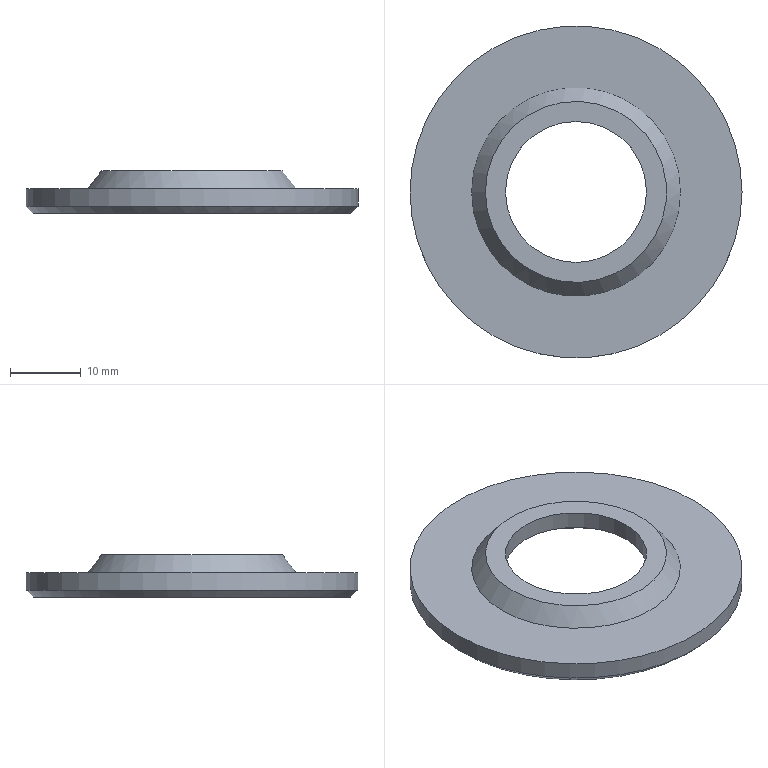Part | NX | features DATUM_CSYS 2, CHAMFER 1, SKETCH 1, SWP104 1 | 1 solid | 9 faces | box 47.08 x 47.08 x 6 mm | volume 4835 mm3 | plane 4 | cone 3 | cylinder 2 | commonest cylinder face diameters 20 x1 47.08 x1
STEP:
#1=CARTESIAN_POINT('',(-10.,0.,0.));
#2=VERTEX_POINT('',#1);
#3=CARTESIAN_POINT('',(0.,0.,0.));
#4=DIRECTION('',(0.,0.,-1.));
#5=DIRECTION('',(-1.,0.,0.));
#6=AXIS2_PLACEMENT_3D('',#3,#4,#5);
#7=CIRCLE('',#6,10.);
#8=EDGE_CURVE('',#2,#2,#7,.T.);
#9=ORIENTED_EDGE('',*,*,#8,.T.);
#10=EDGE_LOOP('',(#9));
#11=FACE_BOUND('',#10,.T.);
#12=CARTESIAN_POINT('',(-12.84,0.,0.));
#13=VERTEX_POINT('',#12);
#14=CARTESIAN_POINT('',(0.,0.,0.));
#15=DIRECTION('',(0.,0.,-1.));
#16=DIRECTION('',(-1.,0.,0.));
#17=AXIS2_PLACEMENT_3D('',#14,#15,#16);
#18=CIRCLE('',#17,12.84);
#19=EDGE_CURVE('',#13,#13,#18,.T.);
#20=ORIENTED_EDGE('',*,*,#19,.F.);
#21=EDGE_LOOP('',(#20));
#22=FACE_BOUND('',#21,.T.);
#23=CARTESIAN_POINT('',(0.,12.84,0.));
#24=DIRECTION('',(0.,0.,1.));
#25=DIRECTION('',(1.,0.,0.));
#26=AXIS2_PLACEMENT_3D('',#23,#24,#25);
#27=PLANE('',#26);
#28=ADVANCED_FACE('',(#11,#22),#27,.T.);
#29=CARTESIAN_POINT('',(-10.,0.,-2.52));
#30=VERTEX_POINT('',#29);
#31=CARTESIAN_POINT('',(0.,0.,-2.52));
#32=DIRECTION('',(0.,0.,-1.));
#33=DIRECTION('',(-1.,0.,0.));
#34=AXIS2_PLACEMENT_3D('',#31,#32,#33);
#35=CIRCLE('',#34,10.);
#36=EDGE_CURVE('',#30,#30,#35,.T.);
#37=ORIENTED_EDGE('',*,*,#36,.T.);
#38=EDGE_LOOP('',(#37));
#39=FACE_BOUND('',#38,.T.);
#40=ORIENTED_EDGE('',*,*,#8,.F.);
#41=EDGE_LOOP('',(#40));
#42=FACE_BOUND('',#41,.T.);
#43=CARTESIAN_POINT('',(0.,0.,0.));
#44=DIRECTION('',(0.,0.,-1.));
#45=DIRECTION('',(-1.,0.,0.));
#46=AXIS2_PLACEMENT_3D('',#43,#44,#45);
#47=CYLINDRICAL_SURFACE('',#46,10.);
#48=ADVANCED_FACE('',(#39,#42),#47,.F.);
#49=CARTESIAN_POINT('',(-11.3,0.,-2.52));
#50=VERTEX_POINT('',#49);
#51=CARTESIAN_POINT('',(0.,0.,-2.52));
#52=DIRECTION('',(0.,0.,-1.));
#53=DIRECTION('',(-1.,0.,0.));
#54=AXIS2_PLACEMENT_3D('',#51,#52,#53);
#55=CIRCLE('',#54,11.3);
#56=EDGE_CURVE('',#50,#50,#55,.T.);
#57=ORIENTED_EDGE('',*,*,#56,.T.);
#58=EDGE_LOOP('',(#57));
#59=FACE_BOUND('',#58,.T.);
#60=ORIENTED_EDGE('',*,*,#36,.F.);
#61=EDGE_LOOP('',(#60));
#62=FACE_BOUND('',#61,.T.);
#63=CARTESIAN_POINT('',(0.,10.,-2.52));
#64=DIRECTION('',(0.,0.,-1.));
#65=DIRECTION('',(-1.,0.,0.));
#66=AXIS2_PLACEMENT_3D('',#63,#64,#65);
#67=PLANE('',#66);
#68=ADVANCED_FACE('',(#59,#62),#67,.T.);
#69=CARTESIAN_POINT('',(-14.8,0.,-6.));
#70=VERTEX_POINT('',#69);
#71=CARTESIAN_POINT('',(0.,0.,-6.));
#72=DIRECTION('',(0.,0.,-1.));
#73=DIRECTION('',(-1.,0.,0.));
#74=AXIS2_PLACEMENT_3D('',#71,#72,#73);
#75=CIRCLE('',#74,14.8);
#76=EDGE_CURVE('',#70,#70,#75,.T.);
#77=ORIENTED_EDGE('',*,*,#76,.T.);
#78=EDGE_LOOP('',(#77));
#79=FACE_BOUND('',#78,.T.);
#80=ORIENTED_EDGE('',*,*,#56,.F.);
#81=EDGE_LOOP('',(#80));
#82=FACE_BOUND('',#81,.T.);
#83=CARTESIAN_POINT('',(0.,0.,-2.52));
#84=DIRECTION('',(0.,0.,-1.));
#85=DIRECTION('',(-1.,0.,0.));
#86=AXIS2_PLACEMENT_3D('',#83,#84,#85);
#87=CONICAL_SURFACE('',#86,11.3,0.7883);
#88=ADVANCED_FACE('',(#79,#82),#87,.F.);
#89=CARTESIAN_POINT('',(-22.54,0.,-6.));
#90=VERTEX_POINT('',#89);
#91=CARTESIAN_POINT('',(0.,0.,-6.));
#92=DIRECTION('',(0.,0.,-1.));
#93=DIRECTION('',(-1.,0.,0.));
#94=AXIS2_PLACEMENT_3D('',#91,#92,#93);
#95=CIRCLE('',#94,22.54);
#96=EDGE_CURVE('',#90,#90,#95,.T.);
#97=ORIENTED_EDGE('',*,*,#96,.T.);
#98=EDGE_LOOP('',(#97));
#99=FACE_BOUND('',#98,.T.);
#100=ORIENTED_EDGE('',*,*,#76,.F.);
#101=EDGE_LOOP('',(#100));
#102=FACE_BOUND('',#101,.T.);
#103=CARTESIAN_POINT('',(0.,14.8,-6.));
#104=DIRECTION('',(0.,0.,-1.));
#105=DIRECTION('',(-1.,0.,0.));
#106=AXIS2_PLACEMENT_3D('',#103,#104,#105);
#107=PLANE('',#106);
#108=ADVANCED_FACE('',(#99,#102),#107,.T.);
#109=CARTESIAN_POINT('',(-23.54,0.,-5.));
#110=VERTEX_POINT('',#109);
#111=CARTESIAN_POINT('',(0.,0.,-5.));
#112=DIRECTION('',(0.,0.,-1.));
#113=DIRECTION('',(-1.,0.,0.));
#114=AXIS2_PLACEMENT_3D('',#111,#112,#113);
#115=CIRCLE('',#114,23.54);
#116=EDGE_CURVE('',#110,#110,#115,.F.);
#117=ORIENTED_EDGE('',*,*,#116,.T.);
#118=EDGE_LOOP('',(#117));
#119=FACE_BOUND('',#118,.T.);
#120=CARTESIAN_POINT('',(-23.54,0.,-2.52));
#121=VERTEX_POINT('',#120);
#122=CARTESIAN_POINT('',(0.,0.,-2.52));
#123=DIRECTION('',(0.,0.,-1.));
#124=DIRECTION('',(-1.,0.,0.));
#125=AXIS2_PLACEMENT_3D('',#122,#123,#124);
#126=CIRCLE('',#125,23.54);
#127=EDGE_CURVE('',#121,#121,#126,.T.);
#128=ORIENTED_EDGE('',*,*,#127,.T.);
#129=EDGE_LOOP('',(#128));
#130=FACE_BOUND('',#129,.T.);
#131=CARTESIAN_POINT('',(0.,0.,0.));
#132=DIRECTION('',(0.,0.,-1.));
#133=DIRECTION('',(-1.,0.,0.));
#134=AXIS2_PLACEMENT_3D('',#131,#132,#133);
#135=CYLINDRICAL_SURFACE('',#134,23.54);
#136=ADVANCED_FACE('',(#119,#130),#135,.T.);
#137=CARTESIAN_POINT('',(-14.8,0.,-2.52));
#138=VERTEX_POINT('',#137);
#139=CARTESIAN_POINT('',(0.,0.,-2.52));
#140=DIRECTION('',(0.,0.,-1.));
#141=DIRECTION('',(-1.,0.,0.));
#142=AXIS2_PLACEMENT_3D('',#139,#140,#141);
#143=CIRCLE('',#142,14.8);
#144=EDGE_CURVE('',#138,#138,#143,.T.);
#145=ORIENTED_EDGE('',*,*,#144,.T.);
#146=EDGE_LOOP('',(#145));
#147=FACE_BOUND('',#146,.T.);
#148=ORIENTED_EDGE('',*,*,#127,.F.);
#149=EDGE_LOOP('',(#148));
#150=FACE_BOUND('',#149,.T.);
#151=CARTESIAN_POINT('',(0.,23.54,-2.52));
#152=DIRECTION('',(0.,0.,1.));
#153=DIRECTION('',(1.,0.,0.));
#154=AXIS2_PLACEMENT_3D('',#151,#152,#153);
#155=PLANE('',#154);
#156=ADVANCED_FACE('',(#147,#150),#155,.T.);
#157=ORIENTED_EDGE('',*,*,#19,.T.);
#158=EDGE_LOOP('',(#157));
#159=FACE_BOUND('',#158,.T.);
#160=ORIENTED_EDGE('',*,*,#144,.F.);
#161=EDGE_LOOP('',(#160));
#162=FACE_BOUND('',#161,.T.);
#163=CARTESIAN_POINT('',(0.,0.,-2.52));
#164=DIRECTION('',(0.,0.,-1.));
#165=DIRECTION('',(-1.,0.,0.));
#166=AXIS2_PLACEMENT_3D('',#163,#164,#165);
#167=CONICAL_SURFACE('',#166,14.8,0.661);
#168=ADVANCED_FACE('',(#159,#162),#167,.T.);
#169=ORIENTED_EDGE('',*,*,#116,.F.);
#170=EDGE_LOOP('',(#169));
#171=FACE_BOUND('',#170,.T.);
#172=ORIENTED_EDGE('',*,*,#96,.F.);
#173=EDGE_LOOP('',(#172));
#174=FACE_BOUND('',#173,.T.);
#175=CARTESIAN_POINT('',(0.,0.,-6.));
#176=DIRECTION('',(0.,0.,1.));
#177=DIRECTION('',(1.,0.,0.));
#178=AXIS2_PLACEMENT_3D('',#175,#176,#177);
#179=CONICAL_SURFACE('',#178,22.54,0.7854);
#180=ADVANCED_FACE('',(#171,#174),#179,.T.);
#181=CLOSED_SHELL('',(#28,#48,#68,#88,#108,#136,#156,#168,#180));
#182=MANIFOLD_SOLID_BREP('',#181);
#183=(LENGTH_UNIT()NAMED_UNIT(*)SI_UNIT(.MILLI.,.METRE.));
#184=UNCERTAINTY_MEASURE_WITH_UNIT(LENGTH_MEASURE(0.00001),#183,'','');
#185=(NAMED_UNIT(*)PLANE_ANGLE_UNIT()SI_UNIT($,.RADIAN.));
#186=(NAMED_UNIT(*)SI_UNIT($,.STERADIAN.)SOLID_ANGLE_UNIT());
#187=(GEOMETRIC_REPRESENTATION_CONTEXT(3)GLOBAL_UNCERTAINTY_ASSIGNED_CONTEXT((#184))GLOBAL_UNIT_ASSIGNED_CONTEXT((#183,#185,#186))REPRESENTATION_CONTEXT('',''));
#188=ADVANCED_BREP_SHAPE_REPRESENTATION('',(#182),#187);